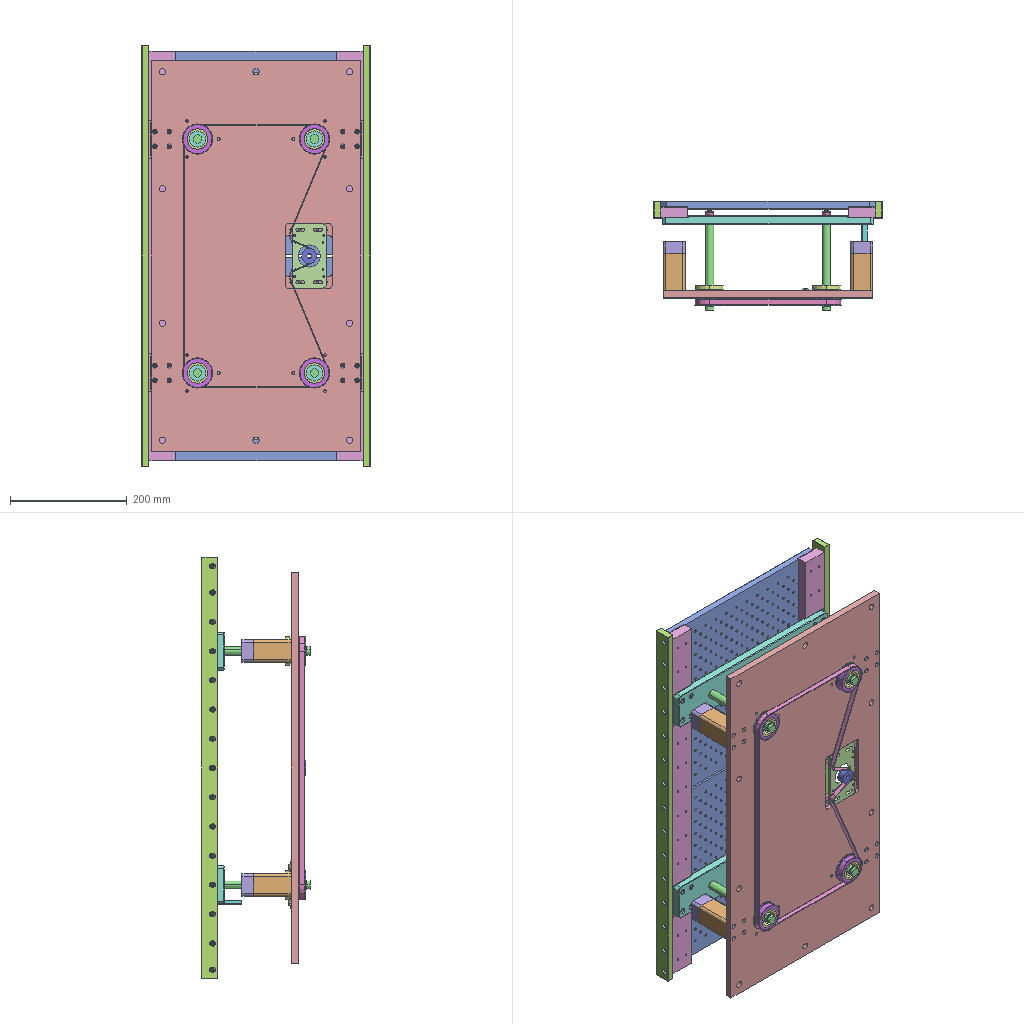Assembly | SolidWorks | 18 different items | 47 placed | box 390 x 186 x 720 mm
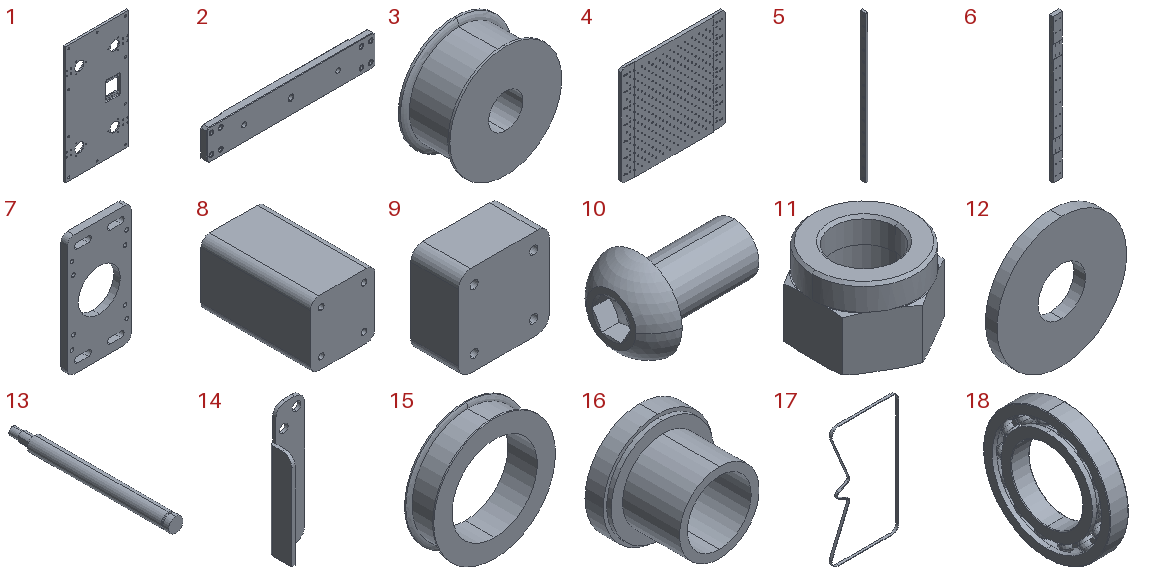Parts list (item | quantity | size | volume | features):
1 | x1 | 359 x 12 x 668 mm | 2636785 mm3 | features ICE 5, HoleWzd 3, Extrusion 1
2 | x2 | 360 x 15 x 65 mm | 330070 mm3 | features HoleWzd 3, ICE 3, Chamfer 2, Extrusion 1
3 | x1 | 26 x 12 x 26 mm | 4546 mm3 | features Revolution 2
4 | x2 | 366 x 12 x 348 mm | 1403273 mm3 | features ICE 2, Chamfer 1, Extrusion 1, HoleWzd 1
5 | x2 | 12 x 28 x 720 mm | 234641 mm3 | features Chamfer 1, Extrusion 1, HoleWzd 1
6 | x2 | 45 x 18 x 700 mm | 549074 mm3 | features HoleWzd 3, Extrusion 1, ICE 1, LPattern 1
7 | x1 | 58 x 6 x 110 mm | 28962 mm3 | features HoleWzd 2, Extrusion 1, ICE 1
8 | x4 | 38 x 64 x 38 mm | 90329 mm3 | features HoleWzd 2, ICE 2, Extrusion 1, Fillet 1
9 | x4 | 38 x 20 x 38 mm | 26957 mm3 | features Extrusion 1, HoleWzd 1
10 | x3 | 15.3 x 10.5 x 10.5 mm | 508.665 mm3 | features RevCut 2, Revolution 2, Cut 1, LPattern 1, RefAxis 1
11 | x4 | 12.74 x 14.38 x 9.5 mm | 787.765 mm3 | features Cut 3, Boss 1, Chamfer 1, Extrusion 1
12 | x3 | 18 x 1.6 x 18 mm | 352.411 mm3 | features Revolution 1
13 | x4 | 15 x 170 x 15 mm | 27374 mm3 | features ICE 1, RevCut 1, Revolution 1
14 | x1 | 10 x 7 x 40 mm | 544.385 mm3 | features ICE 2, Fillet 1, FlatPattern 1, SMBaseFlange 1, SheetMetal 1
15 | x4 | 50 x 12 x 50 mm | 8776 mm3 | features Revolution 2
16 | x4 | 48 x 35 x 48 mm | 19426 mm3 | features HoleWzd 1, Revolution 1
17 | x1 | 248.84 x 9 x 448.84 mm | 19272 mm3 | features Extrusion 1
18 | x4 | 9 x 62 x 62 mm | 13612 mm3 | features Revolution 5, CirPattern 2, RevCut 2
Mates (type | each side: item.copy, entity, surface, feature):
Coincident | 5.1 face plane Boss-Extrude1 | 4.1 face plane Boss-Extrude1 | 2 times
Coincident | 5.1 face plane Boss-Extrude1 | 6.1 face plane Boss-Extrude1
Coincident | 4.1 face plane Cut-Extrude1 | 6.1 face plane Boss-Extrude1
Coincident | 4.1 face plane Cut-Extrude1 | 6.2 face plane Boss-Extrude1
Coincident | 5.2 face plane Boss-Extrude1 | 6.2 face plane Boss-Extrude1
Coincident | 4.1 face plane Boss-Extrude1 | 6.2 face plane Boss-Extrude1
Coincident | 5.2 face plane Boss-Extrude1 | 4.1 face plane Boss-Extrude1 | 2 times
Coincident | 4.2 face plane Boss-Extrude1 | 4.1 face plane Boss-Extrude1
Coincident | 4.2 face plane Boss-Extrude1 | 5.2 face plane Boss-Extrude1
Coincident | 4.2 face plane Boss-Extrude1 | 6.2 face plane Boss-Extrude1
Concentric | 6.2 face cylinder M4 Tapped Hole2 | 2.1 face cylinder Hole size (%based on) socket head cap screw type 1 | 2 times
Coincident | 6.2 face plane Cut-Extrude3 | 2.1 face plane Cut-Extrude1
Coincident | 6.2 face plane Cut-Extrude3 | 2.2 face plane Cut-Extrude1
Concentric | 6.2 face cylinder M4 Tapped Hole2 | 2.2 face cylinder Hole size (%based on) socket head cap screw type 1 | 2 times
Concentric | 4.1 face cylinder Hole size (%based on) socket head cap screw type 1 | 6.1 face cylinder M4 Tapped Hole3
Coincident | 5.1 face plane Boss-Extrude1 | 5.2 face plane Boss-Extrude1
Coincident | 2.1 face plane Boss-Extrude1 | 13.1 face plane Revolve1
Concentric | 13.1 face cylinder Revolve1 | 11.1 face cylinder Base-Extrude1
Parallel | 2.1 face plane Boss-Extrude1 | 13.1 face plane Cut-Extrude1
Concentric | 13.1 face cylinder Revolve1 | 18.1 face cylinder Boss-Revolve3
Coincident | 1.1 face plane Cut-Extrude2 | 18.1 face plane Boss-Revolve3
Concentric | 13.1 face cylinder Revolve1 | 16.1 face cylinder Revolve1
Coincident | 18.1 face plane Boss-Revolve4 | 16.1 face plane Revolve1
Concentric | 16.1 face cylinder Revolve1 | 15.1 face cylinder Revolve1
Coincident | 16.1 face plane Revolve1 | 15.1 face plane Revolve1
Concentric | 1.1 face cylinder M6 Tapped Hole1 | 12.1 face cylinder Base-Revolve1
Coincident | 1.1 face plane Boss-Extrude1 | 12.1 face plane Base-Revolve1
Concentric | 12.1 face cylinder Base-Revolve1 | 10.1 face cylinder Revolve1
Coincident | 12.1 face plane Base-Revolve1 | 10.1 face plane Revolve1
Concentric | 10.2 face cylinder Revolve1 | 12.2 face cylinder Base-Revolve1
Coincident | 10.2 face plane Revolve1 | 12.2 face plane Base-Revolve1
Concentric | 1.1 face cylinder M6 Tapped Hole1 | 12.2 face cylinder Base-Revolve1
Coincident | 1.1 face plane Boss-Extrude1 | 12.2 face plane Base-Revolve1
Concentric | 10.3 face cylinder Revolve1 | 12.3 face cylinder Base-Revolve1
Coincident | 10.3 face plane Revolve1 | 12.3 face plane Base-Revolve1
Concentric | 1.1 face cylinder M6 Tapped Hole1 | 12.3 face cylinder Base-Revolve1
Coincident | 1.1 face plane Boss-Extrude1 | 12.3 face plane Base-Revolve1
Coincident | 2.1 face plane Cut-Extrude3 | 11.1 face plane Base-Extrude1
Concentric | 16.2 face cylinder Revolve1 | 18.2 face cylinder Boss-Revolve4
Coincident | 16.2 face plane Revolve1 | 18.2 face plane Boss-Revolve4
Concentric | 16.2 face cylinder Revolve1 | 13.2 face cylinder Revolve1
Concentric | 13.2 face cylinder Revolve1 | 11.2 face cylinder Base-Extrude1
Coincident | 13.2 face plane Revolve1 | 11.2 face plane Base-Extrude1
Concentric | 16.2 face cylinder Revolve1 | 15.2 face cylinder Revolve1
Coincident | 16.2 face plane Revolve1 | 15.2 face plane Revolve1
Concentric | 1.1 face cylinder Cut-Extrude2 | 18.2 face cylinder Boss-Revolve3
Coincident | 1.1 face plane Cut-Extrude2 | 18.2 face plane Boss-Revolve3
Coincident | 2.1 face plane Cut-Extrude3 | 11.2 face plane Base-Extrude1
Concentric | 16.3 face cylinder Revolve1 | 18.3 face cylinder Boss-Revolve4
Coincident | 16.3 face plane Revolve1 | 18.3 face plane Boss-Revolve4
Concentric | 13.3 face cylinder Revolve1 | 16.3 face cylinder Revolve1
Concentric | 11.3 face cylinder Base-Extrude1 | 13.3 face cylinder Revolve1
Coincident | 11.3 face plane Base-Extrude1 | 13.3 face plane Revolve1
Concentric | 16.3 face cylinder Revolve1 | 15.3 face cylinder Revolve1
Coincident | 16.3 face plane Revolve1 | 15.3 face plane Revolve1
Concentric | 1.1 face cylinder Cut-Extrude2 | 18.3 face cylinder Boss-Revolve3
Coincident | 1.1 face plane Cut-Extrude2 | 18.3 face plane Boss-Revolve3
Coincident | 2.2 face plane Cut-Extrude3 | 11.3 face plane Base-Extrude1
Concentric | 16.4 face cylinder Revolve1 | 18.4 face cylinder Boss-Revolve4
Coincident | 16.4 face plane Revolve1 | 18.4 face plane Boss-Revolve4
Concentric | 13.4 face cylinder Revolve1 | 16.4 face cylinder Revolve1
Concentric | 11.4 face cylinder Base-Extrude1 | 13.4 face cylinder Revolve1
Coincident | 11.4 face plane Base-Extrude1 | 13.4 face plane Revolve1
Concentric | 16.4 face cylinder Revolve1 | 15.4 face cylinder Revolve1
Coincident | 16.4 face plane Revolve1 | 15.4 face plane Revolve1
Concentric | 1.1 face cylinder Cut-Extrude2 | 18.4 face cylinder Boss-Revolve3
Coincident | 1.1 face plane Cut-Extrude2 | 18.4 face plane Boss-Revolve3
Coincident | 2.2 face plane Cut-Extrude3 | 11.4 face plane Base-Extrude1
LimitDistanceDim | 4.1 face plane Boss-Extrude1 | 1.1 face plane Boss-Extrude1
Concentric | 2.2 face cylinder Cut-Extrude2 | 13.4 face cylinder Revolve1
Concentric | 2.1 face cylinder Cut-Extrude2 | 13.2 face cylinder Revolve1
Coincident | 8.1 face plane Boss-Extrude2 | 9.1 face plane Boss-Extrude1
Concentric | 8.1 face cylinder M4 Tapped Hole1 | 9.1 face cylinder Hole size (%based on) socket head cap screw type 1 | 2 times
Concentric | 1.1 face cylinder Hole size (%based on) socket head cap screw type 1 | 8.1 face cylinder M4 Tapped Hole2 | 2 times
Coincident | 1.1 face plane Boss-Extrude1 | 8.1 face plane Boss-Extrude1
Coincident | 8.2 face plane Boss-Extrude2 | 9.2 face plane Boss-Extrude1
Concentric | 8.2 face cylinder M4 Tapped Hole1 | 9.2 face cylinder Hole size (%based on) socket head cap screw type 1 | 2 times
Concentric | 1.1 face cylinder Hole size (%based on) socket head cap screw type 1 | 8.2 face cylinder M4 Tapped Hole2 | 2 times
Coincident | 1.1 face plane Boss-Extrude1 | 8.2 face plane Boss-Extrude1
Coincident | 8.3 face plane Boss-Extrude2 | 9.3 face plane Boss-Extrude1
Concentric | 8.3 face cylinder M4 Tapped Hole1 | 9.3 face cylinder Hole size (%based on) socket head cap screw type 1 | 2 times
Concentric | 1.1 face cylinder Hole size (%based on) socket head cap screw type 1 | 8.3 face cylinder M4 Tapped Hole2 | 2 times
Coincident | 1.1 face plane Boss-Extrude1 | 8.3 face plane Boss-Extrude1
Coincident | 8.4 face plane Boss-Extrude2 | 9.4 face plane Boss-Extrude1
Concentric | 8.4 face cylinder M4 Tapped Hole1 | 9.4 face cylinder Hole size (%based on) socket head cap screw type 1 | 2 times
Concentric | 1.1 face cylinder Hole size (%based on) socket head cap screw type 1 | 8.4 face cylinder M4 Tapped Hole2 | 2 times
Coincident | 1.1 face plane Boss-Extrude1 | 8.4 face plane Boss-Extrude1
Coincident | 15.3 face plane Revolve1 | 3.1 face plane Revolve1
Concentric | 3.1 face cylinder Revolve1 | 7.1 face cylinder Boss-Extrude1
Coincident | 1.1 face plane Cut-Extrude8 | 7.1 face plane Boss-Extrude1 | 2 times
DistanceDim | 1.1 face plane Cut-Extrude6 | 7.1 face plane Boss-Extrude1
Concentric | 3.1 face cylinder Revolve1 | 17.1 face cylinder Boss-Extrude1
Parallel | 1.1 face plane Boss-Extrude1 | 17.1 face plane Boss-Extrude1
DistanceDim | 17.1 face plane Boss-Extrude1 | 15.4 face plane Revolve1
Slot | 6.1 face cylinder M4 Tapped Hole1 | 5.1 face cylinder Hole size (%based on) socket head cap screw type 6
Coincident | 2.1 face plane Boss-Extrude1 | 14.1 face plane Base-Flange1
Coincident | 2.1 face plane Boss-Extrude1 | 14.1 face plane Cut-Extrude1